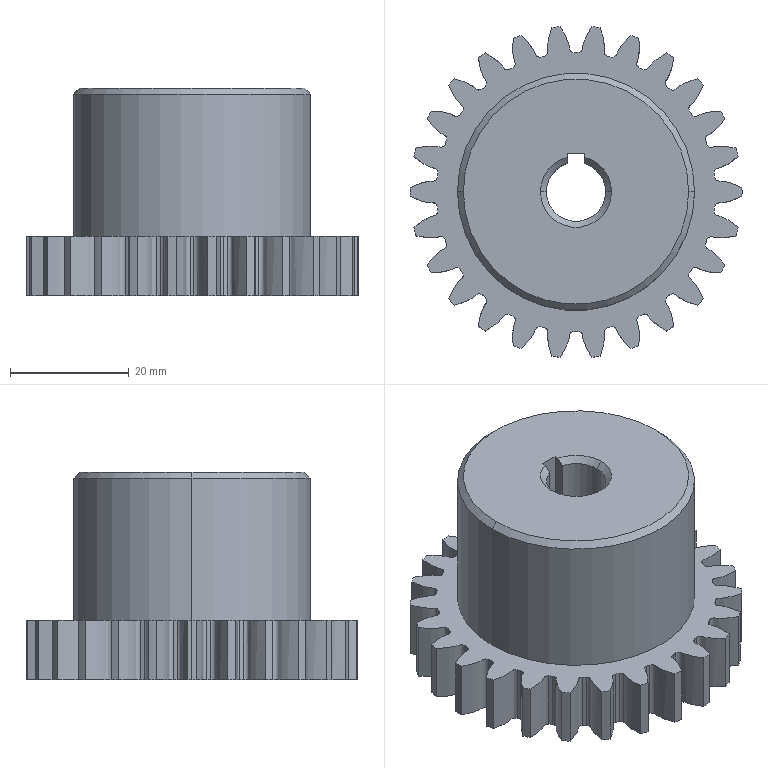Part | SolidWorks | features ICE 4, Chamfer 1, CirPattern 1, Extrusion 1, RefAxis 1 | 1 solid | 124 faces | box 56 x 55.747 x 35 mm | volume 49300 mm3 | cylinder 58 | spline 52 | cone 8 | plane 6 | commonest cylinder face diameters 56 x27 47 x26 10 x3 40 x2